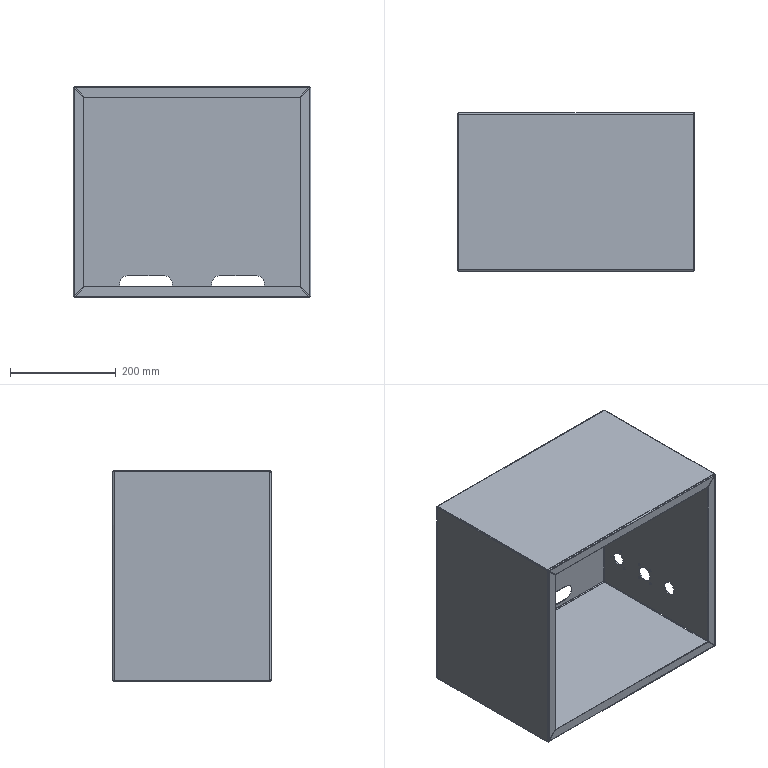Part | STEP file | JBJ-P-1013-06 | 1 solid | 91 faces | box 450 x 300 x 400 mm | volume 843882 mm3 | plane 45 | cylinder 30 | spline 16 | commonest cylinder face diameters 3 x8 5.4 x8 4 x7 30 x4 25 x1 25.7 x1